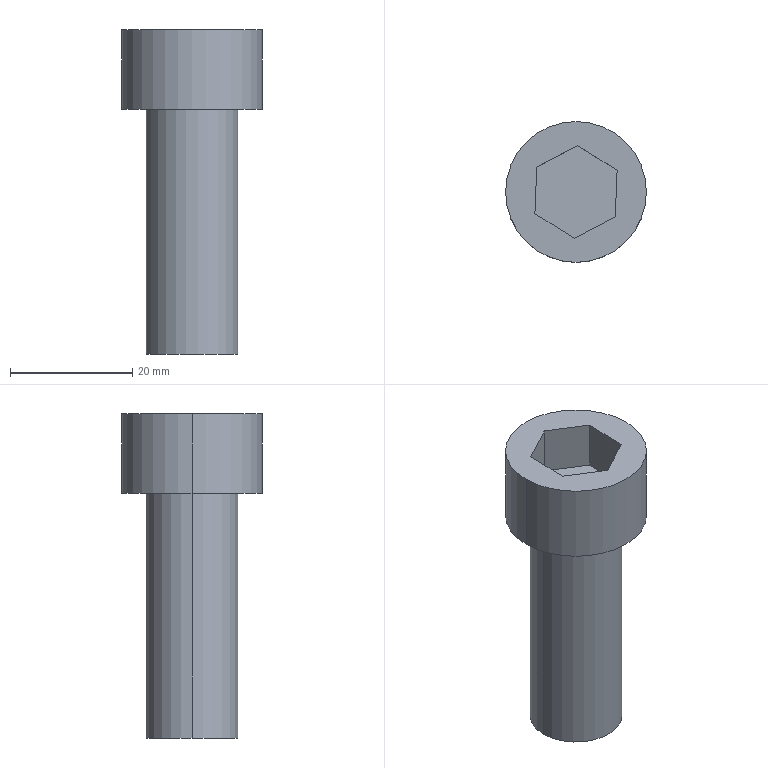Part | SolidWorks | features ICE 2, Extrusion 1 | 1 solid | 14 faces | box 23 x 23 x 53 mm | volume 11275 mm3 | plane 10 | cylinder 4 | commonest cylinder face diameters 15 x2 23 x2
STEP:
#1=CARTESIAN_POINT('',(11.5,0.,53.));
#2=VERTEX_POINT('',#1);
#3=CARTESIAN_POINT('',(-11.5,0.,53.));
#4=VERTEX_POINT('',#3);
#5=CARTESIAN_POINT('',(0.,0.,53.));
#6=DIRECTION('',(0.,0.,1.));
#7=DIRECTION('',(1.,0.,0.));
#8=AXIS2_PLACEMENT_3D('',#5,#6,#7);
#9=CIRCLE('',#8,11.5);
#10=EDGE_CURVE('',#2,#4,#9,.T.);
#11=ORIENTED_EDGE('',*,*,#10,.F.);
#12=CARTESIAN_POINT('',(11.5,0.,40.));
#13=VERTEX_POINT('',#12);
#14=CARTESIAN_POINT('',(11.5,0.,53.));
#15=DIRECTION('',(0.,0.,-1.));
#16=VECTOR('',#15,1000.);
#17=LINE('',#14,#16);
#18=EDGE_CURVE('',#2,#13,#17,.T.);
#19=ORIENTED_EDGE('',*,*,#18,.T.);
#20=CARTESIAN_POINT('',(-11.5,0.,40.));
#21=VERTEX_POINT('',#20);
#22=CARTESIAN_POINT('',(0.,0.,40.));
#23=DIRECTION('',(0.,0.,1.));
#24=DIRECTION('',(1.,0.,0.));
#25=AXIS2_PLACEMENT_3D('',#22,#23,#24);
#26=CIRCLE('',#25,11.5);
#27=EDGE_CURVE('',#13,#21,#26,.T.);
#28=ORIENTED_EDGE('',*,*,#27,.T.);
#29=CARTESIAN_POINT('',(-11.5,0.,53.));
#30=DIRECTION('',(0.,0.,-1.));
#31=VECTOR('',#30,1000.);
#32=LINE('',#29,#31);
#33=EDGE_CURVE('',#4,#21,#32,.T.);
#34=ORIENTED_EDGE('',*,*,#33,.F.);
#35=EDGE_LOOP('',(#11,#19,#28,#34));
#36=FACE_OUTER_BOUND('',#35,.T.);
#37=CARTESIAN_POINT('',(0.,0.,53.));
#38=DIRECTION('',(0.,0.,-1.));
#39=DIRECTION('',(-1.,0.,0.));
#40=AXIS2_PLACEMENT_3D('',#37,#38,#39);
#41=CYLINDRICAL_SURFACE('',#40,11.5);
#42=ADVANCED_FACE('',(#36),#41,.T.);
#43=CARTESIAN_POINT('',(7.5,0.,40.));
#44=VERTEX_POINT('',#43);
#45=CARTESIAN_POINT('',(-7.5,0.,40.));
#46=VERTEX_POINT('',#45);
#47=CARTESIAN_POINT('',(0.,0.,40.));
#48=DIRECTION('',(0.,0.,1.));
#49=DIRECTION('',(1.,0.,0.));
#50=AXIS2_PLACEMENT_3D('',#47,#48,#49);
#51=CIRCLE('',#50,7.5);
#52=EDGE_CURVE('',#44,#46,#51,.T.);
#53=ORIENTED_EDGE('',*,*,#52,.F.);
#54=CARTESIAN_POINT('',(7.5,0.,0.));
#55=VERTEX_POINT('',#54);
#56=CARTESIAN_POINT('',(7.5,0.,40.));
#57=DIRECTION('',(0.,0.,-1.));
#58=VECTOR('',#57,1000.);
#59=LINE('',#56,#58);
#60=EDGE_CURVE('',#44,#55,#59,.T.);
#61=ORIENTED_EDGE('',*,*,#60,.T.);
#62=CARTESIAN_POINT('',(-7.5,0.,0.));
#63=VERTEX_POINT('',#62);
#64=CARTESIAN_POINT('',(0.,0.,0.));
#65=DIRECTION('',(0.,0.,1.));
#66=DIRECTION('',(1.,0.,0.));
#67=AXIS2_PLACEMENT_3D('',#64,#65,#66);
#68=CIRCLE('',#67,7.5);
#69=EDGE_CURVE('',#55,#63,#68,.T.);
#70=ORIENTED_EDGE('',*,*,#69,.T.);
#71=CARTESIAN_POINT('',(-7.5,0.,40.));
#72=DIRECTION('',(0.,0.,-1.));
#73=VECTOR('',#72,1000.);
#74=LINE('',#71,#73);
#75=EDGE_CURVE('',#46,#63,#74,.T.);
#76=ORIENTED_EDGE('',*,*,#75,.F.);
#77=EDGE_LOOP('',(#53,#61,#70,#76));
#78=FACE_OUTER_BOUND('',#77,.T.);
#79=CARTESIAN_POINT('',(0.,0.,40.));
#80=DIRECTION('',(0.,0.,-1.));
#81=DIRECTION('',(-1.,0.,0.));
#82=AXIS2_PLACEMENT_3D('',#79,#80,#81);
#83=CYLINDRICAL_SURFACE('',#82,7.5);
#84=ADVANCED_FACE('',(#78),#83,.T.);
#85=ORIENTED_EDGE('',*,*,#60,.F.);
#86=CARTESIAN_POINT('',(0.,0.,40.));
#87=DIRECTION('',(0.,0.,1.));
#88=DIRECTION('',(1.,0.,0.));
#89=AXIS2_PLACEMENT_3D('',#86,#87,#88);
#90=CIRCLE('',#89,7.5);
#91=EDGE_CURVE('',#46,#44,#90,.T.);
#92=ORIENTED_EDGE('',*,*,#91,.F.);
#93=ORIENTED_EDGE('',*,*,#75,.T.);
#94=CARTESIAN_POINT('',(0.,0.,0.));
#95=DIRECTION('',(0.,0.,1.));
#96=DIRECTION('',(1.,0.,0.));
#97=AXIS2_PLACEMENT_3D('',#94,#95,#96);
#98=CIRCLE('',#97,7.5);
#99=EDGE_CURVE('',#63,#55,#98,.T.);
#100=ORIENTED_EDGE('',*,*,#99,.T.);
#101=EDGE_LOOP('',(#85,#92,#93,#100));
#102=FACE_OUTER_BOUND('',#101,.T.);
#103=CARTESIAN_POINT('',(0.,0.,40.));
#104=DIRECTION('',(0.,0.,-1.));
#105=DIRECTION('',(-1.,0.,0.));
#106=AXIS2_PLACEMENT_3D('',#103,#104,#105);
#107=CYLINDRICAL_SURFACE('',#106,7.5);
#108=ADVANCED_FACE('',(#102),#107,.T.);
#109=ORIENTED_EDGE('',*,*,#99,.F.);
#110=ORIENTED_EDGE('',*,*,#69,.F.);
#111=EDGE_LOOP('',(#109,#110));
#112=FACE_OUTER_BOUND('',#111,.T.);
#113=CARTESIAN_POINT('',(0.,0.,0.));
#114=DIRECTION('',(0.,0.,1.));
#115=DIRECTION('',(1.,0.,0.));
#116=AXIS2_PLACEMENT_3D('',#113,#114,#115);
#117=PLANE('',#116);
#118=ADVANCED_FACE('',(#112),#117,.F.);
#119=ORIENTED_EDGE('',*,*,#18,.F.);
#120=CARTESIAN_POINT('',(0.,0.,53.));
#121=DIRECTION('',(0.,0.,1.));
#122=DIRECTION('',(1.,0.,0.));
#123=AXIS2_PLACEMENT_3D('',#120,#121,#122);
#124=CIRCLE('',#123,11.5);
#125=EDGE_CURVE('',#4,#2,#124,.T.);
#126=ORIENTED_EDGE('',*,*,#125,.F.);
#127=ORIENTED_EDGE('',*,*,#33,.T.);
#128=CARTESIAN_POINT('',(0.,0.,40.));
#129=DIRECTION('',(0.,0.,1.));
#130=DIRECTION('',(1.,0.,0.));
#131=AXIS2_PLACEMENT_3D('',#128,#129,#130);
#132=CIRCLE('',#131,11.5);
#133=EDGE_CURVE('',#21,#13,#132,.T.);
#134=ORIENTED_EDGE('',*,*,#133,.T.);
#135=EDGE_LOOP('',(#119,#126,#127,#134));
#136=FACE_OUTER_BOUND('',#135,.T.);
#137=CARTESIAN_POINT('',(0.,0.,53.));
#138=DIRECTION('',(0.,0.,-1.));
#139=DIRECTION('',(-1.,0.,0.));
#140=AXIS2_PLACEMENT_3D('',#137,#138,#139);
#141=CYLINDRICAL_SURFACE('',#140,11.5);
#142=ADVANCED_FACE('',(#136),#141,.T.);
#143=CARTESIAN_POINT('',(-0.2996,-7.577,53.));
#144=VERTEX_POINT('',#143);
#145=CARTESIAN_POINT('',(6.412,-4.048,53.));
#146=VERTEX_POINT('',#145);
#147=CARTESIAN_POINT('',(-0.2996,-7.577,53.));
#148=DIRECTION('',(0.8851,0.4654,0.));
#149=VECTOR('',#148,1000.);
#150=LINE('',#147,#149);
#151=EDGE_CURVE('',#144,#146,#150,.T.);
#152=ORIENTED_EDGE('',*,*,#151,.F.);
#153=CARTESIAN_POINT('',(-6.712,-3.529,53.));
#154=VERTEX_POINT('',#153);
#155=CARTESIAN_POINT('',(-6.712,-3.529,53.));
#156=DIRECTION('',(0.8456,-0.5338,0.));
#157=VECTOR('',#156,1000.);
#158=LINE('',#155,#157);
#159=EDGE_CURVE('',#154,#144,#158,.T.);
#160=ORIENTED_EDGE('',*,*,#159,.F.);
#161=CARTESIAN_POINT('',(-6.412,4.048,53.));
#162=VERTEX_POINT('',#161);
#163=CARTESIAN_POINT('',(-6.412,4.048,53.));
#164=DIRECTION('',(-0.03951,-0.9992,0.));
#165=VECTOR('',#164,1000.);
#166=LINE('',#163,#165);
#167=EDGE_CURVE('',#162,#154,#166,.T.);
#168=ORIENTED_EDGE('',*,*,#167,.F.);
#169=CARTESIAN_POINT('',(0.2996,7.577,53.));
#170=VERTEX_POINT('',#169);
#171=CARTESIAN_POINT('',(0.2996,7.577,53.));
#172=DIRECTION('',(-0.8851,-0.4654,0.));
#173=VECTOR('',#172,1000.);
#174=LINE('',#171,#173);
#175=EDGE_CURVE('',#170,#162,#174,.T.);
#176=ORIENTED_EDGE('',*,*,#175,.F.);
#177=CARTESIAN_POINT('',(6.712,3.529,53.));
#178=VERTEX_POINT('',#177);
#179=CARTESIAN_POINT('',(6.712,3.529,53.));
#180=DIRECTION('',(-0.8456,0.5338,0.));
#181=VECTOR('',#180,1000.);
#182=LINE('',#179,#181);
#183=EDGE_CURVE('',#178,#170,#182,.T.);
#184=ORIENTED_EDGE('',*,*,#183,.F.);
#185=CARTESIAN_POINT('',(6.412,-4.048,53.));
#186=DIRECTION('',(0.03951,0.9992,0.));
#187=VECTOR('',#186,1000.);
#188=LINE('',#185,#187);
#189=EDGE_CURVE('',#146,#178,#188,.T.);
#190=ORIENTED_EDGE('',*,*,#189,.F.);
#191=EDGE_LOOP('',(#152,#160,#168,#176,#184,#190));
#192=FACE_BOUND('',#191,.T.);
#193=ORIENTED_EDGE('',*,*,#125,.T.);
#194=ORIENTED_EDGE('',*,*,#10,.T.);
#195=EDGE_LOOP('',(#193,#194));
#196=FACE_OUTER_BOUND('',#195,.T.);
#197=CARTESIAN_POINT('',(0.,0.,53.));
#198=DIRECTION('',(0.,0.,1.));
#199=DIRECTION('',(1.,0.,0.));
#200=AXIS2_PLACEMENT_3D('',#197,#198,#199);
#201=PLANE('',#200);
#202=ADVANCED_FACE('',(#192,#196),#201,.T.);
#203=ORIENTED_EDGE('',*,*,#91,.T.);
#204=ORIENTED_EDGE('',*,*,#52,.T.);
#205=EDGE_LOOP('',(#203,#204));
#206=FACE_BOUND('',#205,.T.);
#207=ORIENTED_EDGE('',*,*,#133,.F.);
#208=ORIENTED_EDGE('',*,*,#27,.F.);
#209=EDGE_LOOP('',(#207,#208));
#210=FACE_OUTER_BOUND('',#209,.T.);
#211=CARTESIAN_POINT('',(0.,0.,40.));
#212=DIRECTION('',(0.,0.,1.));
#213=DIRECTION('',(1.,0.,0.));
#214=AXIS2_PLACEMENT_3D('',#211,#212,#213);
#215=PLANE('',#214);
#216=ADVANCED_FACE('',(#206,#210),#215,.F.);
#217=ORIENTED_EDGE('',*,*,#151,.T.);
#218=CARTESIAN_POINT('',(6.412,-4.048,45.));
#219=VERTEX_POINT('',#218);
#220=CARTESIAN_POINT('',(6.412,-4.048,45.));
#221=DIRECTION('',(0.,0.,1.));
#222=VECTOR('',#221,1000.);
#223=LINE('',#220,#222);
#224=EDGE_CURVE('',#219,#146,#223,.T.);
#225=ORIENTED_EDGE('',*,*,#224,.F.);
#226=CARTESIAN_POINT('',(-0.2996,-7.577,45.));
#227=VERTEX_POINT('',#226);
#228=CARTESIAN_POINT('',(-0.2996,-7.577,45.));
#229=DIRECTION('',(0.8851,0.4654,0.));
#230=VECTOR('',#229,1000.);
#231=LINE('',#228,#230);
#232=EDGE_CURVE('',#227,#219,#231,.T.);
#233=ORIENTED_EDGE('',*,*,#232,.F.);
#234=CARTESIAN_POINT('',(-0.2996,-7.577,45.));
#235=DIRECTION('',(0.,0.,1.));
#236=VECTOR('',#235,1000.);
#237=LINE('',#234,#236);
#238=EDGE_CURVE('',#227,#144,#237,.T.);
#239=ORIENTED_EDGE('',*,*,#238,.T.);
#240=EDGE_LOOP('',(#217,#225,#233,#239));
#241=FACE_OUTER_BOUND('',#240,.T.);
#242=CARTESIAN_POINT('',(-0.2996,-7.577,45.));
#243=DIRECTION('',(0.4654,-0.8851,0.));
#244=DIRECTION('',(0.8851,0.4654,0.));
#245=AXIS2_PLACEMENT_3D('',#242,#243,#244);
#246=PLANE('',#245);
#247=ADVANCED_FACE('',(#241),#246,.F.);
#248=ORIENTED_EDGE('',*,*,#159,.T.);
#249=ORIENTED_EDGE('',*,*,#238,.F.);
#250=CARTESIAN_POINT('',(-6.712,-3.529,45.));
#251=VERTEX_POINT('',#250);
#252=CARTESIAN_POINT('',(-6.712,-3.529,45.));
#253=DIRECTION('',(0.8456,-0.5338,0.));
#254=VECTOR('',#253,1000.);
#255=LINE('',#252,#254);
#256=EDGE_CURVE('',#251,#227,#255,.T.);
#257=ORIENTED_EDGE('',*,*,#256,.F.);
#258=CARTESIAN_POINT('',(-6.712,-3.529,45.));
#259=DIRECTION('',(0.,0.,1.));
#260=VECTOR('',#259,1000.);
#261=LINE('',#258,#260);
#262=EDGE_CURVE('',#251,#154,#261,.T.);
#263=ORIENTED_EDGE('',*,*,#262,.T.);
#264=EDGE_LOOP('',(#248,#249,#257,#263));
#265=FACE_OUTER_BOUND('',#264,.T.);
#266=CARTESIAN_POINT('',(-6.712,-3.529,45.));
#267=DIRECTION('',(-0.5338,-0.8456,0.));
#268=DIRECTION('',(0.8456,-0.5338,0.));
#269=AXIS2_PLACEMENT_3D('',#266,#267,#268);
#270=PLANE('',#269);
#271=ADVANCED_FACE('',(#265),#270,.F.);
#272=ORIENTED_EDGE('',*,*,#167,.T.);
#273=ORIENTED_EDGE('',*,*,#262,.F.);
#274=CARTESIAN_POINT('',(-6.412,4.048,45.));
#275=VERTEX_POINT('',#274);
#276=CARTESIAN_POINT('',(-6.412,4.048,45.));
#277=DIRECTION('',(-0.03951,-0.9992,0.));
#278=VECTOR('',#277,1000.);
#279=LINE('',#276,#278);
#280=EDGE_CURVE('',#275,#251,#279,.T.);
#281=ORIENTED_EDGE('',*,*,#280,.F.);
#282=CARTESIAN_POINT('',(-6.412,4.048,45.));
#283=DIRECTION('',(0.,0.,1.));
#284=VECTOR('',#283,1000.);
#285=LINE('',#282,#284);
#286=EDGE_CURVE('',#275,#162,#285,.T.);
#287=ORIENTED_EDGE('',*,*,#286,.T.);
#288=EDGE_LOOP('',(#272,#273,#281,#287));
#289=FACE_OUTER_BOUND('',#288,.T.);
#290=CARTESIAN_POINT('',(-6.412,4.048,45.));
#291=DIRECTION('',(-0.9992,0.03951,0.));
#292=DIRECTION('',(-0.03951,-0.9992,0.));
#293=AXIS2_PLACEMENT_3D('',#290,#291,#292);
#294=PLANE('',#293);
#295=ADVANCED_FACE('',(#289),#294,.F.);
#296=ORIENTED_EDGE('',*,*,#175,.T.);
#297=ORIENTED_EDGE('',*,*,#286,.F.);
#298=CARTESIAN_POINT('',(0.2996,7.577,45.));
#299=VERTEX_POINT('',#298);
#300=CARTESIAN_POINT('',(0.2996,7.577,45.));
#301=DIRECTION('',(-0.8851,-0.4654,0.));
#302=VECTOR('',#301,1000.);
#303=LINE('',#300,#302);
#304=EDGE_CURVE('',#299,#275,#303,.T.);
#305=ORIENTED_EDGE('',*,*,#304,.F.);
#306=CARTESIAN_POINT('',(0.2996,7.577,45.));
#307=DIRECTION('',(0.,0.,1.));
#308=VECTOR('',#307,1000.);
#309=LINE('',#306,#308);
#310=EDGE_CURVE('',#299,#170,#309,.T.);
#311=ORIENTED_EDGE('',*,*,#310,.T.);
#312=EDGE_LOOP('',(#296,#297,#305,#311));
#313=FACE_OUTER_BOUND('',#312,.T.);
#314=CARTESIAN_POINT('',(0.2996,7.577,45.));
#315=DIRECTION('',(-0.4654,0.8851,0.));
#316=DIRECTION('',(-0.8851,-0.4654,0.));
#317=AXIS2_PLACEMENT_3D('',#314,#315,#316);
#318=PLANE('',#317);
#319=ADVANCED_FACE('',(#313),#318,.F.);
#320=ORIENTED_EDGE('',*,*,#183,.T.);
#321=ORIENTED_EDGE('',*,*,#310,.F.);
#322=CARTESIAN_POINT('',(6.712,3.529,45.));
#323=VERTEX_POINT('',#322);
#324=CARTESIAN_POINT('',(6.712,3.529,45.));
#325=DIRECTION('',(-0.8456,0.5338,0.));
#326=VECTOR('',#325,1000.);
#327=LINE('',#324,#326);
#328=EDGE_CURVE('',#323,#299,#327,.T.);
#329=ORIENTED_EDGE('',*,*,#328,.F.);
#330=CARTESIAN_POINT('',(6.712,3.529,45.));
#331=DIRECTION('',(0.,0.,1.));
#332=VECTOR('',#331,1000.);
#333=LINE('',#330,#332);
#334=EDGE_CURVE('',#323,#178,#333,.T.);
#335=ORIENTED_EDGE('',*,*,#334,.T.);
#336=EDGE_LOOP('',(#320,#321,#329,#335));
#337=FACE_OUTER_BOUND('',#336,.T.);
#338=CARTESIAN_POINT('',(6.712,3.529,45.));
#339=DIRECTION('',(0.5338,0.8456,0.));
#340=DIRECTION('',(-0.8456,0.5338,0.));
#341=AXIS2_PLACEMENT_3D('',#338,#339,#340);
#342=PLANE('',#341);
#343=ADVANCED_FACE('',(#337),#342,.F.);
#344=ORIENTED_EDGE('',*,*,#189,.T.);
#345=ORIENTED_EDGE('',*,*,#334,.F.);
#346=CARTESIAN_POINT('',(6.412,-4.048,45.));
#347=DIRECTION('',(0.03951,0.9992,0.));
#348=VECTOR('',#347,1000.);
#349=LINE('',#346,#348);
#350=EDGE_CURVE('',#219,#323,#349,.T.);
#351=ORIENTED_EDGE('',*,*,#350,.F.);
#352=ORIENTED_EDGE('',*,*,#224,.T.);
#353=EDGE_LOOP('',(#344,#345,#351,#352));
#354=FACE_OUTER_BOUND('',#353,.T.);
#355=CARTESIAN_POINT('',(6.412,-4.048,45.));
#356=DIRECTION('',(0.9992,-0.03951,0.));
#357=DIRECTION('',(0.03951,0.9992,0.));
#358=AXIS2_PLACEMENT_3D('',#355,#356,#357);
#359=PLANE('',#358);
#360=ADVANCED_FACE('',(#354),#359,.F.);
#361=ORIENTED_EDGE('',*,*,#232,.T.);
#362=ORIENTED_EDGE('',*,*,#350,.T.);
#363=ORIENTED_EDGE('',*,*,#328,.T.);
#364=ORIENTED_EDGE('',*,*,#304,.T.);
#365=ORIENTED_EDGE('',*,*,#280,.T.);
#366=ORIENTED_EDGE('',*,*,#256,.T.);
#367=EDGE_LOOP('',(#361,#362,#363,#364,#365,#366));
#368=FACE_OUTER_BOUND('',#367,.T.);
#369=CARTESIAN_POINT('',(0.,0.,45.));
#370=DIRECTION('',(0.,0.,1.));
#371=DIRECTION('',(1.,0.,0.));
#372=AXIS2_PLACEMENT_3D('',#369,#370,#371);
#373=PLANE('',#372);
#374=ADVANCED_FACE('',(#368),#373,.T.);
#375=CLOSED_SHELL('',(#42,#84,#108,#118,#142,#202,#216,#247,#271,#295,#319,#343,#360,#374));
#376=MANIFOLD_SOLID_BREP('',#375);
#377=CARTESIAN_POINT('',(0.,0.,0.));
#378=DIRECTION('',(0.,0.,1.));
#379=DIRECTION('',(1.,0.,0.));
#380=AXIS2_PLACEMENT_3D('',#377,#378,#379);
#381=(LENGTH_UNIT()NAMED_UNIT(*)SI_UNIT(.MILLI.,.METRE.));
#382=UNCERTAINTY_MEASURE_WITH_UNIT(LENGTH_MEASURE(0.00001),#381,'','');
#383=(NAMED_UNIT(*)PLANE_ANGLE_UNIT()SI_UNIT($,.RADIAN.));
#384=(NAMED_UNIT(*)SI_UNIT($,.STERADIAN.)SOLID_ANGLE_UNIT());
#385=(GEOMETRIC_REPRESENTATION_CONTEXT(3)GLOBAL_UNCERTAINTY_ASSIGNED_CONTEXT((#382))GLOBAL_UNIT_ASSIGNED_CONTEXT((#381,#383,#384))REPRESENTATION_CONTEXT('',''));
#386=ADVANCED_BREP_SHAPE_REPRESENTATION('',(#376,#380),#385);